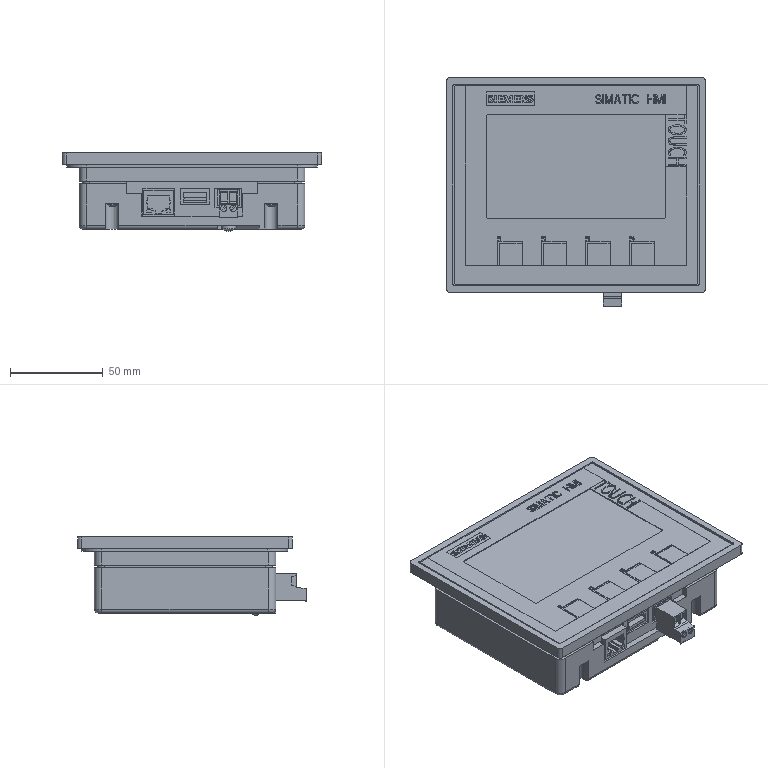Part | NX | features BREP 100 | 100 solids | 1785 faces | box 140 x 123.5 x 42.2 mm | volume 502451 mm3 | plane 1394 | cylinder 217 | spline 159 | cone 10 | torus 4 | sphere 1 | commonest cylinder face diameters 0.4 x52 8 x14 4 x12 5.6 x12 0.5 x8 0.899 x8